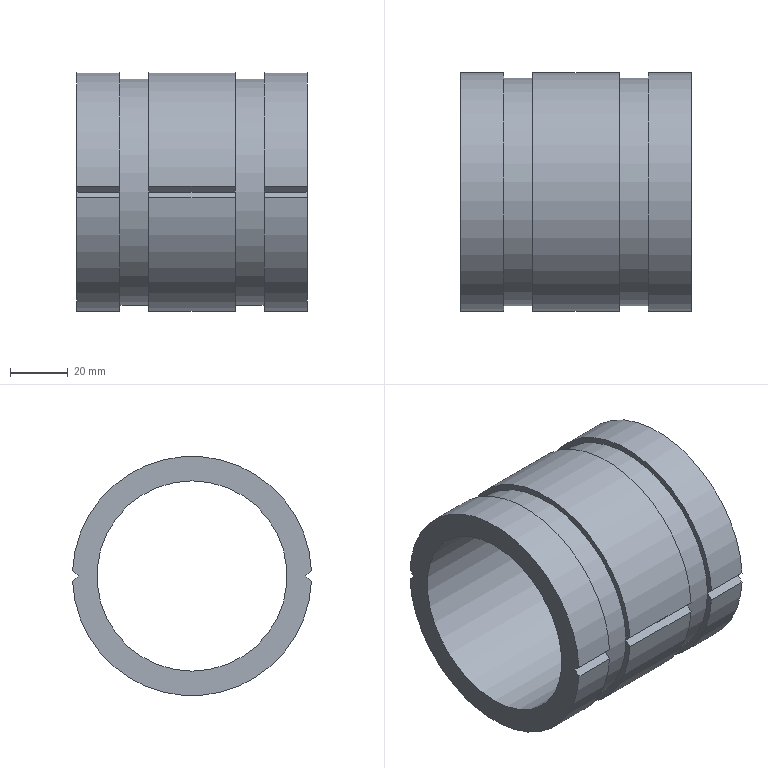Part | NX | features solid 2 | 1 solid | 31 faces | box 80 x 82.908 x 83 mm | volume 148502 mm3 | plane 22 | cylinder 9 | commonest cylinder face diameters 83 x6 79 x2 66 x1
STEP:
#1=CARTESIAN_POINT('',(1415.,-715.,123.));
#2=VERTEX_POINT('',#1);
#3=CARTESIAN_POINT('',(1415.,-715.,90.));
#4=DIRECTION('',(1.,0.,0.));
#5=DIRECTION('',(0.,0.,1.));
#6=AXIS2_PLACEMENT_3D('',#3,#4,#5);
#7=CIRCLE('',#6,33.);
#8=EDGE_CURVE('',#2,#2,#7,.F.);
#9=ORIENTED_EDGE('',*,*,#8,.T.);
#10=EDGE_LOOP('',(#9));
#11=FACE_BOUND('',#10,.T.);
#12=CARTESIAN_POINT('',(1415.,-675.5,90.));
#13=VERTEX_POINT('',#12);
#14=CARTESIAN_POINT('',(1415.,-673.546,91.954));
#15=VERTEX_POINT('',#14);
#16=CARTESIAN_POINT('',(1415.,-711.75,53.75));
#17=DIRECTION('',(0.,0.7071,0.7071));
#18=VECTOR('',#17,1000.);
#19=LINE('',#16,#18);
#20=EDGE_CURVE('',#13,#15,#19,.T.);
#21=ORIENTED_EDGE('',*,*,#20,.T.);
#22=CARTESIAN_POINT('',(1415.,-756.454,91.954));
#23=VERTEX_POINT('',#22);
#24=CARTESIAN_POINT('',(1415.,-715.,90.));
#25=DIRECTION('',(1.,0.,0.));
#26=DIRECTION('',(0.,0.,1.));
#27=AXIS2_PLACEMENT_3D('',#24,#25,#26);
#28=CIRCLE('',#27,41.5);
#29=EDGE_CURVE('',#23,#15,#28,.F.);
#30=ORIENTED_EDGE('',*,*,#29,.F.);
#31=CARTESIAN_POINT('',(1415.,-754.5,90.));
#32=VERTEX_POINT('',#31);
#33=CARTESIAN_POINT('',(1415.,-751.25,86.75));
#34=DIRECTION('',(0.,-0.7071,0.7071));
#35=VECTOR('',#34,1000.);
#36=LINE('',#33,#35);
#37=EDGE_CURVE('',#32,#23,#36,.T.);
#38=ORIENTED_EDGE('',*,*,#37,.F.);
#39=CARTESIAN_POINT('',(1415.,-756.454,88.046));
#40=VERTEX_POINT('',#39);
#41=CARTESIAN_POINT('',(1415.,-751.25,93.25));
#42=DIRECTION('',(0.,0.7071,0.7071));
#43=VECTOR('',#42,1000.);
#44=LINE('',#41,#43);
#45=EDGE_CURVE('',#40,#32,#44,.T.);
#46=ORIENTED_EDGE('',*,*,#45,.F.);
#47=CARTESIAN_POINT('',(1415.,-673.546,88.046));
#48=VERTEX_POINT('',#47);
#49=CARTESIAN_POINT('',(1415.,-715.,90.));
#50=DIRECTION('',(1.,0.,0.));
#51=DIRECTION('',(0.,0.,1.));
#52=AXIS2_PLACEMENT_3D('',#49,#50,#51);
#53=CIRCLE('',#52,41.5);
#54=EDGE_CURVE('',#48,#40,#53,.F.);
#55=ORIENTED_EDGE('',*,*,#54,.F.);
#56=CARTESIAN_POINT('',(1415.,-711.75,126.25));
#57=DIRECTION('',(0.,-0.7071,0.7071));
#58=VECTOR('',#57,1000.);
#59=LINE('',#56,#58);
#60=EDGE_CURVE('',#48,#13,#59,.T.);
#61=ORIENTED_EDGE('',*,*,#60,.T.);
#62=EDGE_LOOP('',(#21,#30,#38,#46,#55,#61));
#63=FACE_BOUND('',#62,.T.);
#64=CARTESIAN_POINT('',(1415.,-748.,90.));
#65=DIRECTION('',(-1.,0.,0.));
#66=DIRECTION('',(0.,0.,-1.));
#67=AXIS2_PLACEMENT_3D('',#64,#65,#66);
#68=PLANE('',#67);
#69=ADVANCED_FACE('',(#11,#63),#68,.F.);
#70=CARTESIAN_POINT('',(1400.,-673.546,91.954));
#71=VERTEX_POINT('',#70);
#72=CARTESIAN_POINT('',(1445.2,-673.546,91.954));
#73=DIRECTION('',(-1.,0.,0.));
#74=VECTOR('',#73,1000.);
#75=LINE('',#72,#74);
#76=EDGE_CURVE('',#71,#15,#75,.F.);
#77=ORIENTED_EDGE('',*,*,#76,.F.);
#78=CARTESIAN_POINT('',(1400.,-756.454,91.954));
#79=VERTEX_POINT('',#78);
#80=CARTESIAN_POINT('',(1400.,-715.,90.));
#81=DIRECTION('',(-1.,0.,0.));
#82=DIRECTION('',(0.,0.,-1.));
#83=AXIS2_PLACEMENT_3D('',#80,#81,#82);
#84=CIRCLE('',#83,41.5);
#85=EDGE_CURVE('',#79,#71,#84,.T.);
#86=ORIENTED_EDGE('',*,*,#85,.F.);
#87=CARTESIAN_POINT('',(1445.2,-756.454,91.954));
#88=DIRECTION('',(-1.,0.,0.));
#89=VECTOR('',#88,1000.);
#90=LINE('',#87,#89);
#91=EDGE_CURVE('',#79,#23,#90,.F.);
#92=ORIENTED_EDGE('',*,*,#91,.T.);
#93=ORIENTED_EDGE('',*,*,#29,.T.);
#94=EDGE_LOOP('',(#77,#86,#92,#93));
#95=FACE_BOUND('',#94,.T.);
#96=CARTESIAN_POINT('',(1445.2,-715.,90.));
#97=DIRECTION('',(-1.,0.,0.));
#98=DIRECTION('',(0.,0.,-1.));
#99=AXIS2_PLACEMENT_3D('',#96,#97,#98);
#100=CYLINDRICAL_SURFACE('',#99,41.5);
#101=ADVANCED_FACE('',(#95),#100,.T.);
#102=CARTESIAN_POINT('',(1400.,-673.546,88.046));
#103=VERTEX_POINT('',#102);
#104=CARTESIAN_POINT('',(1445.2,-673.546,88.046));
#105=DIRECTION('',(-1.,0.,0.));
#106=VECTOR('',#105,1000.);
#107=LINE('',#104,#106);
#108=EDGE_CURVE('',#48,#103,#107,.T.);
#109=ORIENTED_EDGE('',*,*,#108,.F.);
#110=ORIENTED_EDGE('',*,*,#54,.T.);
#111=CARTESIAN_POINT('',(1400.,-756.454,88.046));
#112=VERTEX_POINT('',#111);
#113=CARTESIAN_POINT('',(1445.2,-756.454,88.046));
#114=DIRECTION('',(-1.,0.,0.));
#115=VECTOR('',#114,1000.);
#116=LINE('',#113,#115);
#117=EDGE_CURVE('',#40,#112,#116,.T.);
#118=ORIENTED_EDGE('',*,*,#117,.T.);
#119=CARTESIAN_POINT('',(1400.,-715.,90.));
#120=DIRECTION('',(-1.,0.,0.));
#121=DIRECTION('',(0.,0.,-1.));
#122=AXIS2_PLACEMENT_3D('',#119,#120,#121);
#123=CIRCLE('',#122,41.5);
#124=EDGE_CURVE('',#103,#112,#123,.T.);
#125=ORIENTED_EDGE('',*,*,#124,.F.);
#126=EDGE_LOOP('',(#109,#110,#118,#125));
#127=FACE_BOUND('',#126,.T.);
#128=CARTESIAN_POINT('',(1445.2,-715.,90.));
#129=DIRECTION('',(-1.,0.,0.));
#130=DIRECTION('',(0.,0.,-1.));
#131=AXIS2_PLACEMENT_3D('',#128,#129,#130);
#132=CYLINDRICAL_SURFACE('',#131,41.5);
#133=ADVANCED_FACE('',(#127),#132,.T.);
#134=CARTESIAN_POINT('',(1400.,-675.5,90.));
#135=VERTEX_POINT('',#134);
#136=CARTESIAN_POINT('',(1400.,-675.5,90.));
#137=DIRECTION('',(0.,0.7071,0.7071));
#138=VECTOR('',#137,1000.);
#139=LINE('',#136,#138);
#140=EDGE_CURVE('',#135,#71,#139,.T.);
#141=ORIENTED_EDGE('',*,*,#140,.F.);
#142=CARTESIAN_POINT('',(1400.,-754.5,90.));
#143=VERTEX_POINT('',#142);
#144=CARTESIAN_POINT('',(1400.,-715.,90.));
#145=DIRECTION('',(-1.,0.,0.));
#146=DIRECTION('',(0.,0.,-1.));
#147=AXIS2_PLACEMENT_3D('',#144,#145,#146);
#148=CIRCLE('',#147,39.5);
#149=EDGE_CURVE('',#143,#135,#148,.T.);
#150=ORIENTED_EDGE('',*,*,#149,.F.);
#151=CARTESIAN_POINT('',(1400.,-754.5,90.));
#152=DIRECTION('',(0.,-0.7071,0.7071));
#153=VECTOR('',#152,1000.);
#154=LINE('',#151,#153);
#155=EDGE_CURVE('',#143,#79,#154,.T.);
#156=ORIENTED_EDGE('',*,*,#155,.T.);
#157=ORIENTED_EDGE('',*,*,#85,.T.);
#158=EDGE_LOOP('',(#141,#150,#156,#157));
#159=FACE_BOUND('',#158,.T.);
#160=CARTESIAN_POINT('',(1400.,-756.5,90.));
#161=DIRECTION('',(1.,0.,0.));
#162=DIRECTION('',(0.,0.,1.));
#163=AXIS2_PLACEMENT_3D('',#160,#161,#162);
#164=PLANE('',#163);
#165=ADVANCED_FACE('',(#159),#164,.F.);
#166=CARTESIAN_POINT('',(1400.,-665.5,80.));
#167=DIRECTION('',(0.,-0.7071,0.7071));
#168=VECTOR('',#167,1000.);
#169=LINE('',#166,#168);
#170=EDGE_CURVE('',#103,#135,#169,.T.);
#171=ORIENTED_EDGE('',*,*,#170,.F.);
#172=ORIENTED_EDGE('',*,*,#124,.T.);
#173=CARTESIAN_POINT('',(1400.,-764.5,80.));
#174=DIRECTION('',(0.,0.7071,0.7071));
#175=VECTOR('',#174,1000.);
#176=LINE('',#173,#175);
#177=EDGE_CURVE('',#112,#143,#176,.T.);
#178=ORIENTED_EDGE('',*,*,#177,.T.);
#179=CARTESIAN_POINT('',(1400.,-715.,90.));
#180=DIRECTION('',(-1.,0.,0.));
#181=DIRECTION('',(0.,0.,-1.));
#182=AXIS2_PLACEMENT_3D('',#179,#180,#181);
#183=CIRCLE('',#182,39.5);
#184=EDGE_CURVE('',#135,#143,#183,.T.);
#185=ORIENTED_EDGE('',*,*,#184,.F.);
#186=EDGE_LOOP('',(#171,#172,#178,#185));
#187=FACE_BOUND('',#186,.T.);
#188=CARTESIAN_POINT('',(1400.,-756.5,90.));
#189=DIRECTION('',(1.,0.,0.));
#190=DIRECTION('',(0.,0.,1.));
#191=AXIS2_PLACEMENT_3D('',#188,#189,#190);
#192=PLANE('',#191);
#193=ADVANCED_FACE('',(#187),#192,.F.);
#194=CARTESIAN_POINT('',(1390.,-673.546,91.954));
#195=VERTEX_POINT('',#194);
#196=CARTESIAN_POINT('',(1390.,-675.5,90.));
#197=VERTEX_POINT('',#196);
#198=CARTESIAN_POINT('',(1390.,-675.5,90.));
#199=DIRECTION('',(0.,-0.7071,-0.7071));
#200=VECTOR('',#199,1000.);
#201=LINE('',#198,#200);
#202=EDGE_CURVE('',#195,#197,#201,.T.);
#203=ORIENTED_EDGE('',*,*,#202,.F.);
#204=CARTESIAN_POINT('',(1390.,-756.454,91.954));
#205=VERTEX_POINT('',#204);
#206=CARTESIAN_POINT('',(1390.,-715.,90.));
#207=DIRECTION('',(1.,0.,0.));
#208=DIRECTION('',(0.,0.,1.));
#209=AXIS2_PLACEMENT_3D('',#206,#207,#208);
#210=CIRCLE('',#209,41.5);
#211=EDGE_CURVE('',#205,#195,#210,.F.);
#212=ORIENTED_EDGE('',*,*,#211,.F.);
#213=CARTESIAN_POINT('',(1390.,-754.5,90.));
#214=VERTEX_POINT('',#213);
#215=CARTESIAN_POINT('',(1390.,-754.5,90.));
#216=DIRECTION('',(0.,0.7071,-0.7071));
#217=VECTOR('',#216,1000.);
#218=LINE('',#215,#217);
#219=EDGE_CURVE('',#205,#214,#218,.T.);
#220=ORIENTED_EDGE('',*,*,#219,.T.);
#221=CARTESIAN_POINT('',(1390.,-715.,90.));
#222=DIRECTION('',(1.,0.,0.));
#223=DIRECTION('',(0.,0.,1.));
#224=AXIS2_PLACEMENT_3D('',#221,#222,#223);
#225=CIRCLE('',#224,39.5);
#226=EDGE_CURVE('',#214,#197,#225,.F.);
#227=ORIENTED_EDGE('',*,*,#226,.T.);
#228=EDGE_LOOP('',(#203,#212,#220,#227));
#229=FACE_BOUND('',#228,.T.);
#230=CARTESIAN_POINT('',(1390.,-754.5,90.));
#231=DIRECTION('',(-1.,0.,0.));
#232=DIRECTION('',(0.,0.,-1.));
#233=AXIS2_PLACEMENT_3D('',#230,#231,#232);
#234=PLANE('',#233);
#235=ADVANCED_FACE('',(#229),#234,.F.);
#236=CARTESIAN_POINT('',(1390.,-673.546,88.046));
#237=VERTEX_POINT('',#236);
#238=CARTESIAN_POINT('',(1390.,-665.5,80.));
#239=DIRECTION('',(0.,0.7071,-0.7071));
#240=VECTOR('',#239,1000.);
#241=LINE('',#238,#240);
#242=EDGE_CURVE('',#197,#237,#241,.T.);
#243=ORIENTED_EDGE('',*,*,#242,.F.);
#244=CARTESIAN_POINT('',(1390.,-715.,90.));
#245=DIRECTION('',(1.,0.,0.));
#246=DIRECTION('',(0.,0.,1.));
#247=AXIS2_PLACEMENT_3D('',#244,#245,#246);
#248=CIRCLE('',#247,39.5);
#249=EDGE_CURVE('',#197,#214,#248,.F.);
#250=ORIENTED_EDGE('',*,*,#249,.T.);
#251=CARTESIAN_POINT('',(1390.,-756.454,88.046));
#252=VERTEX_POINT('',#251);
#253=CARTESIAN_POINT('',(1390.,-764.5,80.));
#254=DIRECTION('',(0.,-0.7071,-0.7071));
#255=VECTOR('',#254,1000.);
#256=LINE('',#253,#255);
#257=EDGE_CURVE('',#214,#252,#256,.T.);
#258=ORIENTED_EDGE('',*,*,#257,.T.);
#259=CARTESIAN_POINT('',(1390.,-715.,90.));
#260=DIRECTION('',(1.,0.,0.));
#261=DIRECTION('',(0.,0.,1.));
#262=AXIS2_PLACEMENT_3D('',#259,#260,#261);
#263=CIRCLE('',#262,41.5);
#264=EDGE_CURVE('',#237,#252,#263,.F.);
#265=ORIENTED_EDGE('',*,*,#264,.F.);
#266=EDGE_LOOP('',(#243,#250,#258,#265));
#267=FACE_BOUND('',#266,.T.);
#268=CARTESIAN_POINT('',(1390.,-754.5,90.));
#269=DIRECTION('',(-1.,0.,0.));
#270=DIRECTION('',(0.,0.,-1.));
#271=AXIS2_PLACEMENT_3D('',#268,#269,#270);
#272=PLANE('',#271);
#273=ADVANCED_FACE('',(#267),#272,.F.);
#274=CARTESIAN_POINT('',(1360.,-673.546,91.954));
#275=VERTEX_POINT('',#274);
#276=CARTESIAN_POINT('',(1445.2,-673.546,91.954));
#277=DIRECTION('',(-1.,0.,0.));
#278=VECTOR('',#277,1000.);
#279=LINE('',#276,#278);
#280=EDGE_CURVE('',#275,#195,#279,.F.);
#281=ORIENTED_EDGE('',*,*,#280,.F.);
#282=CARTESIAN_POINT('',(1360.,-756.454,91.954));
#283=VERTEX_POINT('',#282);
#284=CARTESIAN_POINT('',(1360.,-715.,90.));
#285=DIRECTION('',(-1.,0.,0.));
#286=DIRECTION('',(0.,0.,-1.));
#287=AXIS2_PLACEMENT_3D('',#284,#285,#286);
#288=CIRCLE('',#287,41.5);
#289=EDGE_CURVE('',#283,#275,#288,.T.);
#290=ORIENTED_EDGE('',*,*,#289,.F.);
#291=CARTESIAN_POINT('',(1445.2,-756.454,91.954));
#292=DIRECTION('',(-1.,0.,0.));
#293=VECTOR('',#292,1000.);
#294=LINE('',#291,#293);
#295=EDGE_CURVE('',#283,#205,#294,.F.);
#296=ORIENTED_EDGE('',*,*,#295,.T.);
#297=ORIENTED_EDGE('',*,*,#211,.T.);
#298=EDGE_LOOP('',(#281,#290,#296,#297));
#299=FACE_BOUND('',#298,.T.);
#300=CARTESIAN_POINT('',(1445.2,-715.,90.));
#301=DIRECTION('',(-1.,0.,0.));
#302=DIRECTION('',(0.,0.,-1.));
#303=AXIS2_PLACEMENT_3D('',#300,#301,#302);
#304=CYLINDRICAL_SURFACE('',#303,41.5);
#305=ADVANCED_FACE('',(#299),#304,.T.);
#306=CARTESIAN_POINT('',(1360.,-673.546,88.046));
#307=VERTEX_POINT('',#306);
#308=CARTESIAN_POINT('',(1445.2,-673.546,88.046));
#309=DIRECTION('',(-1.,0.,0.));
#310=VECTOR('',#309,1000.);
#311=LINE('',#308,#310);
#312=EDGE_CURVE('',#237,#307,#311,.T.);
#313=ORIENTED_EDGE('',*,*,#312,.F.);
#314=ORIENTED_EDGE('',*,*,#264,.T.);
#315=CARTESIAN_POINT('',(1360.,-756.454,88.046));
#316=VERTEX_POINT('',#315);
#317=CARTESIAN_POINT('',(1445.2,-756.454,88.046));
#318=DIRECTION('',(-1.,0.,0.));
#319=VECTOR('',#318,1000.);
#320=LINE('',#317,#319);
#321=EDGE_CURVE('',#252,#316,#320,.T.);
#322=ORIENTED_EDGE('',*,*,#321,.T.);
#323=CARTESIAN_POINT('',(1360.,-715.,90.));
#324=DIRECTION('',(-1.,0.,0.));
#325=DIRECTION('',(0.,0.,-1.));
#326=AXIS2_PLACEMENT_3D('',#323,#324,#325);
#327=CIRCLE('',#326,41.5);
#328=EDGE_CURVE('',#307,#316,#327,.T.);
#329=ORIENTED_EDGE('',*,*,#328,.F.);
#330=EDGE_LOOP('',(#313,#314,#322,#329));
#331=FACE_BOUND('',#330,.T.);
#332=CARTESIAN_POINT('',(1445.2,-715.,90.));
#333=DIRECTION('',(-1.,0.,0.));
#334=DIRECTION('',(0.,0.,-1.));
#335=AXIS2_PLACEMENT_3D('',#332,#333,#334);
#336=CYLINDRICAL_SURFACE('',#335,41.5);
#337=ADVANCED_FACE('',(#331),#336,.T.);
#338=CARTESIAN_POINT('',(1360.,-675.5,90.));
#339=VERTEX_POINT('',#338);
#340=CARTESIAN_POINT('',(1360.,-675.5,90.));
#341=DIRECTION('',(0.,0.7071,0.7071));
#342=VECTOR('',#341,1000.);
#343=LINE('',#340,#342);
#344=EDGE_CURVE('',#339,#275,#343,.T.);
#345=ORIENTED_EDGE('',*,*,#344,.F.);
#346=CARTESIAN_POINT('',(1360.,-754.5,90.));
#347=VERTEX_POINT('',#346);
#348=CARTESIAN_POINT('',(1360.,-715.,90.));
#349=DIRECTION('',(-1.,0.,0.));
#350=DIRECTION('',(0.,0.,-1.));
#351=AXIS2_PLACEMENT_3D('',#348,#349,#350);
#352=CIRCLE('',#351,39.5);
#353=EDGE_CURVE('',#347,#339,#352,.T.);
#354=ORIENTED_EDGE('',*,*,#353,.F.);
#355=CARTESIAN_POINT('',(1360.,-754.5,90.));
#356=DIRECTION('',(0.,-0.7071,0.7071));
#357=VECTOR('',#356,1000.);
#358=LINE('',#355,#357);
#359=EDGE_CURVE('',#347,#283,#358,.T.);
#360=ORIENTED_EDGE('',*,*,#359,.T.);
#361=ORIENTED_EDGE('',*,*,#289,.T.);
#362=EDGE_LOOP('',(#345,#354,#360,#361));
#363=FACE_BOUND('',#362,.T.);
#364=CARTESIAN_POINT('',(1360.,-756.5,90.));
#365=DIRECTION('',(1.,0.,0.));
#366=DIRECTION('',(0.,0.,1.));
#367=AXIS2_PLACEMENT_3D('',#364,#365,#366);
#368=PLANE('',#367);
#369=ADVANCED_FACE('',(#363),#368,.F.);
#370=CARTESIAN_POINT('',(1360.,-665.5,80.));
#371=DIRECTION('',(0.,-0.7071,0.7071));
#372=VECTOR('',#371,1000.);
#373=LINE('',#370,#372);
#374=EDGE_CURVE('',#307,#339,#373,.T.);
#375=ORIENTED_EDGE('',*,*,#374,.F.);
#376=ORIENTED_EDGE('',*,*,#328,.T.);
#377=CARTESIAN_POINT('',(1360.,-764.5,80.));
#378=DIRECTION('',(0.,0.7071,0.7071));
#379=VECTOR('',#378,1000.);
#380=LINE('',#377,#379);
#381=EDGE_CURVE('',#316,#347,#380,.T.);
#382=ORIENTED_EDGE('',*,*,#381,.T.);
#383=CARTESIAN_POINT('',(1360.,-715.,90.));
#384=DIRECTION('',(-1.,0.,0.));
#385=DIRECTION('',(0.,0.,-1.));
#386=AXIS2_PLACEMENT_3D('',#383,#384,#385);
#387=CIRCLE('',#386,39.5);
#388=EDGE_CURVE('',#339,#347,#387,.T.);
#389=ORIENTED_EDGE('',*,*,#388,.F.);
#390=EDGE_LOOP('',(#375,#376,#382,#389));
#391=FACE_BOUND('',#390,.T.);
#392=CARTESIAN_POINT('',(1360.,-756.5,90.));
#393=DIRECTION('',(1.,0.,0.));
#394=DIRECTION('',(0.,0.,1.));
#395=AXIS2_PLACEMENT_3D('',#392,#393,#394);
#396=PLANE('',#395);
#397=ADVANCED_FACE('',(#391),#396,.F.);
#398=CARTESIAN_POINT('',(1350.,-673.546,91.954));
#399=VERTEX_POINT('',#398);
#400=CARTESIAN_POINT('',(1350.,-675.5,90.));
#401=VERTEX_POINT('',#400);
#402=CARTESIAN_POINT('',(1350.,-675.5,90.));
#403=DIRECTION('',(0.,-0.7071,-0.7071));
#404=VECTOR('',#403,1000.);
#405=LINE('',#402,#404);
#406=EDGE_CURVE('',#399,#401,#405,.T.);
#407=ORIENTED_EDGE('',*,*,#406,.F.);
#408=CARTESIAN_POINT('',(1350.,-756.454,91.954));
#409=VERTEX_POINT('',#408);
#410=CARTESIAN_POINT('',(1350.,-715.,90.));
#411=DIRECTION('',(1.,0.,0.));
#412=DIRECTION('',(0.,0.,1.));
#413=AXIS2_PLACEMENT_3D('',#410,#411,#412);
#414=CIRCLE('',#413,41.5);
#415=EDGE_CURVE('',#409,#399,#414,.F.);
#416=ORIENTED_EDGE('',*,*,#415,.F.);
#417=CARTESIAN_POINT('',(1350.,-754.5,90.));
#418=VERTEX_POINT('',#417);
#419=CARTESIAN_POINT('',(1350.,-754.5,90.));
#420=DIRECTION('',(0.,0.7071,-0.7071));
#421=VECTOR('',#420,1000.);
#422=LINE('',#419,#421);
#423=EDGE_CURVE('',#409,#418,#422,.T.);
#424=ORIENTED_EDGE('',*,*,#423,.T.);
#425=CARTESIAN_POINT('',(1350.,-715.,90.));
#426=DIRECTION('',(1.,0.,0.));
#427=DIRECTION('',(0.,0.,1.));
#428=AXIS2_PLACEMENT_3D('',#425,#426,#427);
#429=CIRCLE('',#428,39.5);
#430=EDGE_CURVE('',#418,#401,#429,.F.);
#431=ORIENTED_EDGE('',*,*,#430,.T.);
#432=EDGE_LOOP('',(#407,#416,#424,#431));
#433=FACE_BOUND('',#432,.T.);
#434=CARTESIAN_POINT('',(1350.,-754.5,90.));
#435=DIRECTION('',(-1.,0.,0.));
#436=DIRECTION('',(0.,0.,-1.));
#437=AXIS2_PLACEMENT_3D('',#434,#435,#436);
#438=PLANE('',#437);
#439=ADVANCED_FACE('',(#433),#438,.F.);
#440=CARTESIAN_POINT('',(1350.,-673.546,88.046));
#441=VERTEX_POINT('',#440);
#442=CARTESIAN_POINT('',(1350.,-665.5,80.));
#443=DIRECTION('',(0.,0.7071,-0.7071));
#444=VECTOR('',#443,1000.);
#445=LINE('',#442,#444);
#446=EDGE_CURVE('',#401,#441,#445,.T.);
#447=ORIENTED_EDGE('',*,*,#446,.F.);
#448=CARTESIAN_POINT('',(1350.,-715.,90.));
#449=DIRECTION('',(1.,0.,0.));
#450=DIRECTION('',(0.,0.,1.));
#451=AXIS2_PLACEMENT_3D('',#448,#449,#450);
#452=CIRCLE('',#451,39.5);
#453=EDGE_CURVE('',#401,#418,#452,.F.);
#454=ORIENTED_EDGE('',*,*,#453,.T.);
#455=CARTESIAN_POINT('',(1350.,-756.454,88.046));
#456=VERTEX_POINT('',#455);
#457=CARTESIAN_POINT('',(1350.,-764.5,80.));
#458=DIRECTION('',(0.,-0.7071,-0.7071));
#459=VECTOR('',#458,1000.);
#460=LINE('',#457,#459);
#461=EDGE_CURVE('',#418,#456,#460,.T.);
#462=ORIENTED_EDGE('',*,*,#461,.T.);
#463=CARTESIAN_POINT('',(1350.,-715.,90.));
#464=DIRECTION('',(1.,0.,0.));
#465=DIRECTION('',(0.,0.,1.));
#466=AXIS2_PLACEMENT_3D('',#463,#464,#465);
#467=CIRCLE('',#466,41.5);
#468=EDGE_CURVE('',#441,#456,#467,.F.);
#469=ORIENTED_EDGE('',*,*,#468,.F.);
#470=EDGE_LOOP('',(#447,#454,#462,#469));
#471=FACE_BOUND('',#470,.T.);
#472=CARTESIAN_POINT('',(1350.,-754.5,90.));
#473=DIRECTION('',(-1.,0.,0.));
#474=DIRECTION('',(0.,0.,-1.));
#475=AXIS2_PLACEMENT_3D('',#472,#473,#474);
#476=PLANE('',#475);
#477=ADVANCED_FACE('',(#471),#476,.F.);
#478=CARTESIAN_POINT('',(1335.,-673.546,91.954));
#479=VERTEX_POINT('',#478);
#480=CARTESIAN_POINT('',(1445.2,-673.546,91.954));
#481=DIRECTION('',(-1.,0.,0.));
#482=VECTOR('',#481,1000.);
#483=LINE('',#480,#482);
#484=EDGE_CURVE('',#479,#399,#483,.F.);
#485=ORIENTED_EDGE('',*,*,#484,.F.);
#486=CARTESIAN_POINT('',(1335.,-756.454,91.954));
#487=VERTEX_POINT('',#486);
#488=CARTESIAN_POINT('',(1335.,-715.,90.));
#489=DIRECTION('',(-1.,0.,0.));
#490=DIRECTION('',(0.,0.,-1.));
#491=AXIS2_PLACEMENT_3D('',#488,#489,#490);
#492=CIRCLE('',#491,41.5);
#493=EDGE_CURVE('',#487,#479,#492,.T.);
#494=ORIENTED_EDGE('',*,*,#493,.F.);
#495=CARTESIAN_POINT('',(1445.2,-756.454,91.954));
#496=DIRECTION('',(-1.,0.,0.));
#497=VECTOR('',#496,1000.);
#498=LINE('',#495,#497);
#499=EDGE_CURVE('',#487,#409,#498,.F.);
#500=ORIENTED_EDGE('',*,*,#499,.T.);
#501=ORIENTED_EDGE('',*,*,#415,.T.);
#502=EDGE_LOOP('',(#485,#494,#500,#501));
#503=FACE_BOUND('',#502,.T.);
#504=CARTESIAN_POINT('',(1445.2,-715.,90.));
#505=DIRECTION('',(-1.,0.,0.));
#506=DIRECTION('',(0.,0.,-1.));
#507=AXIS2_PLACEMENT_3D('',#504,#505,#506);
#508=CYLINDRICAL_SURFACE('',#507,41.5);
#509=ADVANCED_FACE('',(#503),#508,.T.);
#510=CARTESIAN_POINT('',(1335.,-673.546,88.046));
#511=VERTEX_POINT('',#510);
#512=CARTESIAN_POINT('',(1445.2,-673.546,88.046));
#513=DIRECTION('',(-1.,0.,0.));
#514=VECTOR('',#513,1000.);
#515=LINE('',#512,#514);
#516=EDGE_CURVE('',#441,#511,#515,.T.);
#517=ORIENTED_EDGE('',*,*,#516,.F.);
#518=ORIENTED_EDGE('',*,*,#468,.T.);
#519=CARTESIAN_POINT('',(1335.,-756.454,88.046));
#520=VERTEX_POINT('',#519);
#521=CARTESIAN_POINT('',(1445.2,-756.454,88.046));
#522=DIRECTION('',(-1.,0.,0.));
#523=VECTOR('',#522,1000.);
#524=LINE('',#521,#523);
#525=EDGE_CURVE('',#456,#520,#524,.T.);
#526=ORIENTED_EDGE('',*,*,#525,.T.);
#527=CARTESIAN_POINT('',(1335.,-715.,90.));
#528=DIRECTION('',(-1.,0.,0.));
#529=DIRECTION('',(0.,0.,-1.));
#530=AXIS2_PLACEMENT_3D('',#527,#528,#529);
#531=CIRCLE('',#530,41.5);
#532=EDGE_CURVE('',#511,#520,#531,.T.);
#533=ORIENTED_EDGE('',*,*,#532,.F.);
#534=EDGE_LOOP('',(#517,#518,#526,#533));
#535=FACE_BOUND('',#534,.T.);
#536=CARTESIAN_POINT('',(1445.2,-715.,90.));
#537=DIRECTION('',(-1.,0.,0.));
#538=DIRECTION('',(0.,0.,-1.));
#539=AXIS2_PLACEMENT_3D('',#536,#537,#538);
#540=CYLINDRICAL_SURFACE('',#539,41.5);
#541=ADVANCED_FACE('',(#535),#540,.T.);
#542=CARTESIAN_POINT('',(1335.,-715.,57.));
#543=VERTEX_POINT('',#542);
#544=CARTESIAN_POINT('',(1335.,-715.,90.));
#545=DIRECTION('',(-1.,0.,0.));
#546=DIRECTION('',(0.,0.,-1.));
#547=AXIS2_PLACEMENT_3D('',#544,#545,#546);
#548=CIRCLE('',#547,33.);
#549=EDGE_CURVE('',#543,#543,#548,.T.);
#550=ORIENTED_EDGE('',*,*,#549,.F.);
#551=EDGE_LOOP('',(#550));
#552=FACE_BOUND('',#551,.T.);
#553=CARTESIAN_POINT('',(1335.,-675.5,90.));
#554=VERTEX_POINT('',#553);
#555=CARTESIAN_POINT('',(1335.,-675.5,90.));
#556=DIRECTION('',(0.,0.7071,0.7071));
#557=VECTOR('',#556,1000.);
#558=LINE('',#555,#557);
#559=EDGE_CURVE('',#554,#479,#558,.T.);
#560=ORIENTED_EDGE('',*,*,#559,.F.);
#561=CARTESIAN_POINT('',(1335.,-665.5,80.));
#562=DIRECTION('',(0.,-0.7071,0.7071));
#563=VECTOR('',#562,1000.);
#564=LINE('',#561,#563);
#565=EDGE_CURVE('',#511,#554,#564,.T.);
#566=ORIENTED_EDGE('',*,*,#565,.F.);
#567=ORIENTED_EDGE('',*,*,#532,.T.);
#568=CARTESIAN_POINT('',(1335.,-754.5,90.));
#569=VERTEX_POINT('',#568);
#570=CARTESIAN_POINT('',(1335.,-764.5,80.));
#571=DIRECTION('',(0.,0.7071,0.7071));
#572=VECTOR('',#571,1000.);
#573=LINE('',#570,#572);
#574=EDGE_CURVE('',#520,#569,#573,.T.);
#575=ORIENTED_EDGE('',*,*,#574,.T.);
#576=CARTESIAN_POINT('',(1335.,-754.5,90.));
#577=DIRECTION('',(0.,-0.7071,0.7071));
#578=VECTOR('',#577,1000.);
#579=LINE('',#576,#578);
#580=EDGE_CURVE('',#569,#487,#579,.T.);
#581=ORIENTED_EDGE('',*,*,#580,.T.);
#582=ORIENTED_EDGE('',*,*,#493,.T.);
#583=EDGE_LOOP('',(#560,#566,#567,#575,#581,#582));
#584=FACE_BOUND('',#583,.T.);
#585=CARTESIAN_POINT('',(1335.,-756.5,90.));
#586=DIRECTION('',(1.,0.,0.));
#587=DIRECTION('',(0.,0.,1.));
#588=AXIS2_PLACEMENT_3D('',#585,#586,#587);
#589=PLANE('',#588);
#590=ADVANCED_FACE('',(#552,#584),#589,.F.);
#591=ORIENTED_EDGE('',*,*,#249,.F.);
#592=ORIENTED_EDGE('',*,*,#226,.F.);
#593=EDGE_LOOP('',(#591,#592));
#594=FACE_BOUND('',#593,.T.);
#595=ORIENTED_EDGE('',*,*,#149,.T.);
#596=ORIENTED_EDGE('',*,*,#184,.T.);
#597=EDGE_LOOP('',(#595,#596));
#598=FACE_BOUND('',#597,.T.);
#599=CARTESIAN_POINT('',(1445.2,-715.,90.));
#600=DIRECTION('',(-1.,0.,0.));
#601=DIRECTION('',(0.,0.,-1.));
#602=AXIS2_PLACEMENT_3D('',#599,#600,#601);
#603=CYLINDRICAL_SURFACE('',#602,39.5);
#604=ADVANCED_FACE('',(#594,#598),#603,.T.);
#605=ORIENTED_EDGE('',*,*,#453,.F.);
#606=ORIENTED_EDGE('',*,*,#430,.F.);
#607=EDGE_LOOP('',(#605,#606));
#608=FACE_BOUND('',#607,.T.);
#609=ORIENTED_EDGE('',*,*,#353,.T.);
#610=ORIENTED_EDGE('',*,*,#388,.T.);
#611=EDGE_LOOP('',(#609,#610));
#612=FACE_BOUND('',#611,.T.);
#613=CARTESIAN_POINT('',(1445.2,-715.,90.));
#614=DIRECTION('',(-1.,0.,0.));
#615=DIRECTION('',(0.,0.,-1.));
#616=AXIS2_PLACEMENT_3D('',#613,#614,#615);
#617=CYLINDRICAL_SURFACE('',#616,39.5);
#618=ADVANCED_FACE('',(#608,#612),#617,.T.);
#619=ORIENTED_EDGE('',*,*,#549,.T.);
#620=EDGE_LOOP('',(#619));
#621=FACE_BOUND('',#620,.T.);
#622=ORIENTED_EDGE('',*,*,#8,.F.);
#623=EDGE_LOOP('',(#622));
#624=FACE_BOUND('',#623,.T.);
#625=CARTESIAN_POINT('',(1445.2,-715.,90.));
#626=DIRECTION('',(-1.,0.,0.));
#627=DIRECTION('',(0.,0.,-1.));
#628=AXIS2_PLACEMENT_3D('',#625,#626,#627);
#629=CYLINDRICAL_SURFACE('',#628,33.);
#630=ADVANCED_FACE('',(#621,#624),#629,.F.);
#631=ORIENTED_EDGE('',*,*,#499,.F.);
#632=ORIENTED_EDGE('',*,*,#580,.F.);
#633=CARTESIAN_POINT('',(1325.,-754.5,90.));
#634=DIRECTION('',(1.,0.,0.));
#635=VECTOR('',#634,1000.);
#636=LINE('',#633,#635);
#637=EDGE_CURVE('',#569,#418,#636,.T.);
#638=ORIENTED_EDGE('',*,*,#637,.T.);
#639=ORIENTED_EDGE('',*,*,#423,.F.);
#640=EDGE_LOOP('',(#631,#632,#638,#639));
#641=FACE_BOUND('',#640,.T.);
#642=CARTESIAN_POINT('',(1325.,-754.5,90.));
#643=DIRECTION('',(0.,0.7071,0.7071));
#644=DIRECTION('',(0.,0.7071,-0.7071));
#645=AXIS2_PLACEMENT_3D('',#642,#643,#644);
#646=PLANE('',#645);
#647=ADVANCED_FACE('',(#641),#646,.F.);
#648=ORIENTED_EDGE('',*,*,#637,.F.);
#649=ORIENTED_EDGE('',*,*,#574,.F.);
#650=ORIENTED_EDGE('',*,*,#525,.F.);
#651=ORIENTED_EDGE('',*,*,#461,.F.);
#652=EDGE_LOOP('',(#648,#649,#650,#651));
#653=FACE_BOUND('',#652,.T.);
#654=CARTESIAN_POINT('',(1325.,-764.5,80.));
#655=DIRECTION('',(0.,0.7071,-0.7071));
#656=DIRECTION('',(0.,-0.7071,-0.7071));
#657=AXIS2_PLACEMENT_3D('',#654,#655,#656);
#658=PLANE('',#657);
#659=ADVANCED_FACE('',(#653),#658,.F.);
#660=ORIENTED_EDGE('',*,*,#295,.F.);
#661=ORIENTED_EDGE('',*,*,#359,.F.);
#662=CARTESIAN_POINT('',(1325.,-754.5,90.));
#663=DIRECTION('',(1.,0.,0.));
#664=VECTOR('',#663,1000.);
#665=LINE('',#662,#664);
#666=EDGE_CURVE('',#347,#214,#665,.T.);
#667=ORIENTED_EDGE('',*,*,#666,.T.);
#668=ORIENTED_EDGE('',*,*,#219,.F.);
#669=EDGE_LOOP('',(#660,#661,#667,#668));
#670=FACE_BOUND('',#669,.T.);
#671=CARTESIAN_POINT('',(1325.,-754.5,90.));
#672=DIRECTION('',(0.,0.7071,0.7071));
#673=DIRECTION('',(0.,0.7071,-0.7071));
#674=AXIS2_PLACEMENT_3D('',#671,#672,#673);
#675=PLANE('',#674);
#676=ADVANCED_FACE('',(#670),#675,.F.);
#677=ORIENTED_EDGE('',*,*,#666,.F.);
#678=ORIENTED_EDGE('',*,*,#381,.F.);
#679=ORIENTED_EDGE('',*,*,#321,.F.);
#680=ORIENTED_EDGE('',*,*,#257,.F.);
#681=EDGE_LOOP('',(#677,#678,#679,#680));
#682=FACE_BOUND('',#681,.T.);
#683=CARTESIAN_POINT('',(1325.,-764.5,80.));
#684=DIRECTION('',(0.,0.7071,-0.7071));
#685=DIRECTION('',(0.,-0.7071,-0.7071));
#686=AXIS2_PLACEMENT_3D('',#683,#684,#685);
#687=PLANE('',#686);
#688=ADVANCED_FACE('',(#682),#687,.F.);
#689=ORIENTED_EDGE('',*,*,#45,.T.);
#690=CARTESIAN_POINT('',(1325.,-754.5,90.));
#691=DIRECTION('',(1.,0.,0.));
#692=VECTOR('',#691,1000.);
#693=LINE('',#690,#692);
#694=EDGE_CURVE('',#143,#32,#693,.T.);
#695=ORIENTED_EDGE('',*,*,#694,.F.);
#696=ORIENTED_EDGE('',*,*,#177,.F.);
#697=ORIENTED_EDGE('',*,*,#117,.F.);
#698=EDGE_LOOP('',(#689,#695,#696,#697));
#699=FACE_BOUND('',#698,.T.);
#700=CARTESIAN_POINT('',(1325.,-764.5,80.));
#701=DIRECTION('',(0.,0.7071,-0.7071));
#702=DIRECTION('',(0.,-0.7071,-0.7071));
#703=AXIS2_PLACEMENT_3D('',#700,#701,#702);
#704=PLANE('',#703);
#705=ADVANCED_FACE('',(#699),#704,.F.);
#706=ORIENTED_EDGE('',*,*,#155,.F.);
#707=ORIENTED_EDGE('',*,*,#694,.T.);
#708=ORIENTED_EDGE('',*,*,#37,.T.);
#709=ORIENTED_EDGE('',*,*,#91,.F.);
#710=EDGE_LOOP('',(#706,#707,#708,#709));
#711=FACE_BOUND('',#710,.T.);
#712=CARTESIAN_POINT('',(1325.,-754.5,90.));
#713=DIRECTION('',(0.,0.7071,0.7071));
#714=DIRECTION('',(0.,0.7071,-0.7071));
#715=AXIS2_PLACEMENT_3D('',#712,#713,#714);
#716=PLANE('',#715);
#717=ADVANCED_FACE('',(#711),#716,.F.);
#718=ORIENTED_EDGE('',*,*,#446,.T.);
#719=ORIENTED_EDGE('',*,*,#516,.T.);
#720=ORIENTED_EDGE('',*,*,#565,.T.);
#721=CARTESIAN_POINT('',(1325.,-675.5,90.));
#722=DIRECTION('',(1.,0.,0.));
#723=VECTOR('',#722,1000.);
#724=LINE('',#721,#723);
#725=EDGE_CURVE('',#554,#401,#724,.T.);
#726=ORIENTED_EDGE('',*,*,#725,.T.);
#727=EDGE_LOOP('',(#718,#719,#720,#726));
#728=FACE_BOUND('',#727,.T.);
#729=CARTESIAN_POINT('',(1325.,-665.5,80.));
#730=DIRECTION('',(0.,0.7071,0.7071));
#731=DIRECTION('',(0.,0.7071,-0.7071));
#732=AXIS2_PLACEMENT_3D('',#729,#730,#731);
#733=PLANE('',#732);
#734=ADVANCED_FACE('',(#728),#733,.T.);
#735=ORIENTED_EDGE('',*,*,#406,.T.);
#736=ORIENTED_EDGE('',*,*,#725,.F.);
#737=ORIENTED_EDGE('',*,*,#559,.T.);
#738=ORIENTED_EDGE('',*,*,#484,.T.);
#739=EDGE_LOOP('',(#735,#736,#737,#738));
#740=FACE_BOUND('',#739,.T.);
#741=CARTESIAN_POINT('',(1325.,-675.5,90.));
#742=DIRECTION('',(0.,0.7071,-0.7071));
#743=DIRECTION('',(0.,-0.7071,-0.7071));
#744=AXIS2_PLACEMENT_3D('',#741,#742,#743);
#745=PLANE('',#744);
#746=ADVANCED_FACE('',(#740),#745,.T.);
#747=ORIENTED_EDGE('',*,*,#242,.T.);
#748=ORIENTED_EDGE('',*,*,#312,.T.);
#749=ORIENTED_EDGE('',*,*,#374,.T.);
#750=CARTESIAN_POINT('',(1325.,-675.5,90.));
#751=DIRECTION('',(1.,0.,0.));
#752=VECTOR('',#751,1000.);
#753=LINE('',#750,#752);
#754=EDGE_CURVE('',#339,#197,#753,.T.);
#755=ORIENTED_EDGE('',*,*,#754,.T.);
#756=EDGE_LOOP('',(#747,#748,#749,#755));
#757=FACE_BOUND('',#756,.T.);
#758=CARTESIAN_POINT('',(1325.,-665.5,80.));
#759=DIRECTION('',(0.,0.7071,0.7071));
#760=DIRECTION('',(0.,0.7071,-0.7071));
#761=AXIS2_PLACEMENT_3D('',#758,#759,#760);
#762=PLANE('',#761);
#763=ADVANCED_FACE('',(#757),#762,.T.);
#764=ORIENTED_EDGE('',*,*,#202,.T.);
#765=ORIENTED_EDGE('',*,*,#754,.F.);
#766=ORIENTED_EDGE('',*,*,#344,.T.);
#767=ORIENTED_EDGE('',*,*,#280,.T.);
#768=EDGE_LOOP('',(#764,#765,#766,#767));
#769=FACE_BOUND('',#768,.T.);
#770=CARTESIAN_POINT('',(1325.,-675.5,90.));
#771=DIRECTION('',(0.,0.7071,-0.7071));
#772=DIRECTION('',(0.,-0.7071,-0.7071));
#773=AXIS2_PLACEMENT_3D('',#770,#771,#772);
#774=PLANE('',#773);
#775=ADVANCED_FACE('',(#769),#774,.T.);
#776=ORIENTED_EDGE('',*,*,#76,.T.);
#777=ORIENTED_EDGE('',*,*,#20,.F.);
#778=CARTESIAN_POINT('',(1325.,-675.5,90.));
#779=DIRECTION('',(1.,0.,0.));
#780=VECTOR('',#779,1000.);
#781=LINE('',#778,#780);
#782=EDGE_CURVE('',#135,#13,#781,.T.);
#783=ORIENTED_EDGE('',*,*,#782,.F.);
#784=ORIENTED_EDGE('',*,*,#140,.T.);
#785=EDGE_LOOP('',(#776,#777,#783,#784));
#786=FACE_BOUND('',#785,.T.);
#787=CARTESIAN_POINT('',(1325.,-675.5,90.));
#788=DIRECTION('',(0.,0.7071,-0.7071));
#789=DIRECTION('',(0.,-0.7071,-0.7071));
#790=AXIS2_PLACEMENT_3D('',#787,#788,#789);
#791=PLANE('',#790);
#792=ADVANCED_FACE('',(#786),#791,.T.);
#793=ORIENTED_EDGE('',*,*,#108,.T.);
#794=ORIENTED_EDGE('',*,*,#170,.T.);
#795=ORIENTED_EDGE('',*,*,#782,.T.);
#796=ORIENTED_EDGE('',*,*,#60,.F.);
#797=EDGE_LOOP('',(#793,#794,#795,#796));
#798=FACE_BOUND('',#797,.T.);
#799=CARTESIAN_POINT('',(1325.,-665.5,80.));
#800=DIRECTION('',(0.,0.7071,0.7071));
#801=DIRECTION('',(0.,0.7071,-0.7071));
#802=AXIS2_PLACEMENT_3D('',#799,#800,#801);
#803=PLANE('',#802);
#804=ADVANCED_FACE('',(#798),#803,.T.);
#805=CLOSED_SHELL('',(#69,#101,#133,#165,#193,#235,#273,#305,#337,#369,#397,#439,#477,#509,#541,#590,#604,#618,#630,#647,#659,#676,#688,#705,#717,#734,#746,#763,#775,#792,#804));
#806=MANIFOLD_SOLID_BREP('',#805);
#807=(LENGTH_UNIT()NAMED_UNIT(*)SI_UNIT(.MILLI.,.METRE.));
#808=UNCERTAINTY_MEASURE_WITH_UNIT(LENGTH_MEASURE(0.00001),#807,'','');
#809=(NAMED_UNIT(*)PLANE_ANGLE_UNIT()SI_UNIT($,.RADIAN.));
#810=(NAMED_UNIT(*)SI_UNIT($,.STERADIAN.)SOLID_ANGLE_UNIT());
#811=(GEOMETRIC_REPRESENTATION_CONTEXT(3)GLOBAL_UNCERTAINTY_ASSIGNED_CONTEXT((#808))GLOBAL_UNIT_ASSIGNED_CONTEXT((#807,#809,#810))REPRESENTATION_CONTEXT('',''));
#812=ADVANCED_BREP_SHAPE_REPRESENTATION('',(#806),#811);